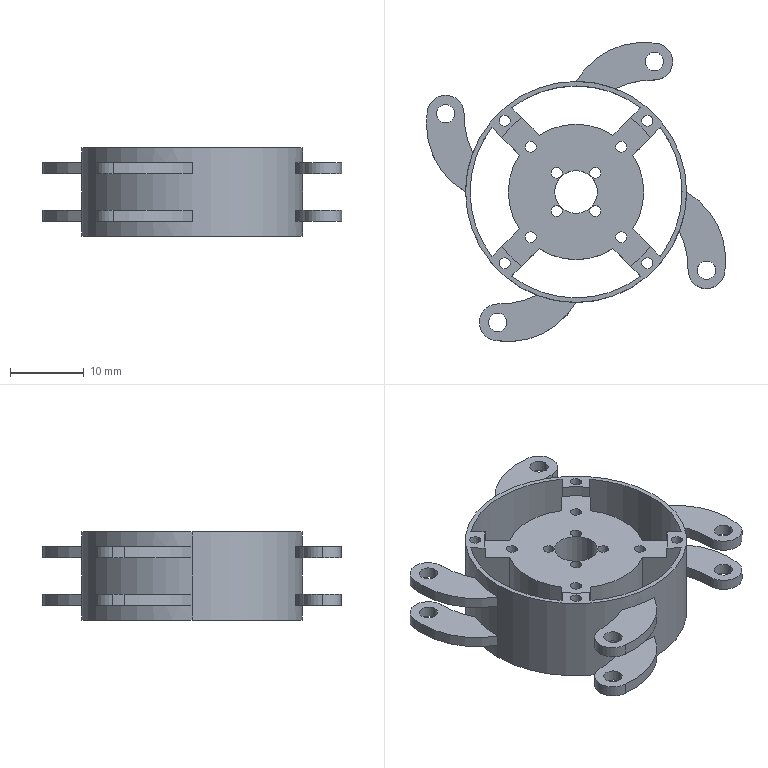Part | SolidWorks | features ICE 6, CirPattern 1, Extrusion 1, MirrorPattern 1, Scale 1 | 1 solid | 122 faces | box 40.64 x 40.64 x 12 mm | volume 4015 mm3 | cylinder 94 | plane 28 | commonest cylinder face diameters 1.5 x24 2.5 x16 5 x12 21.279 x10 23.786 x10 25 x8